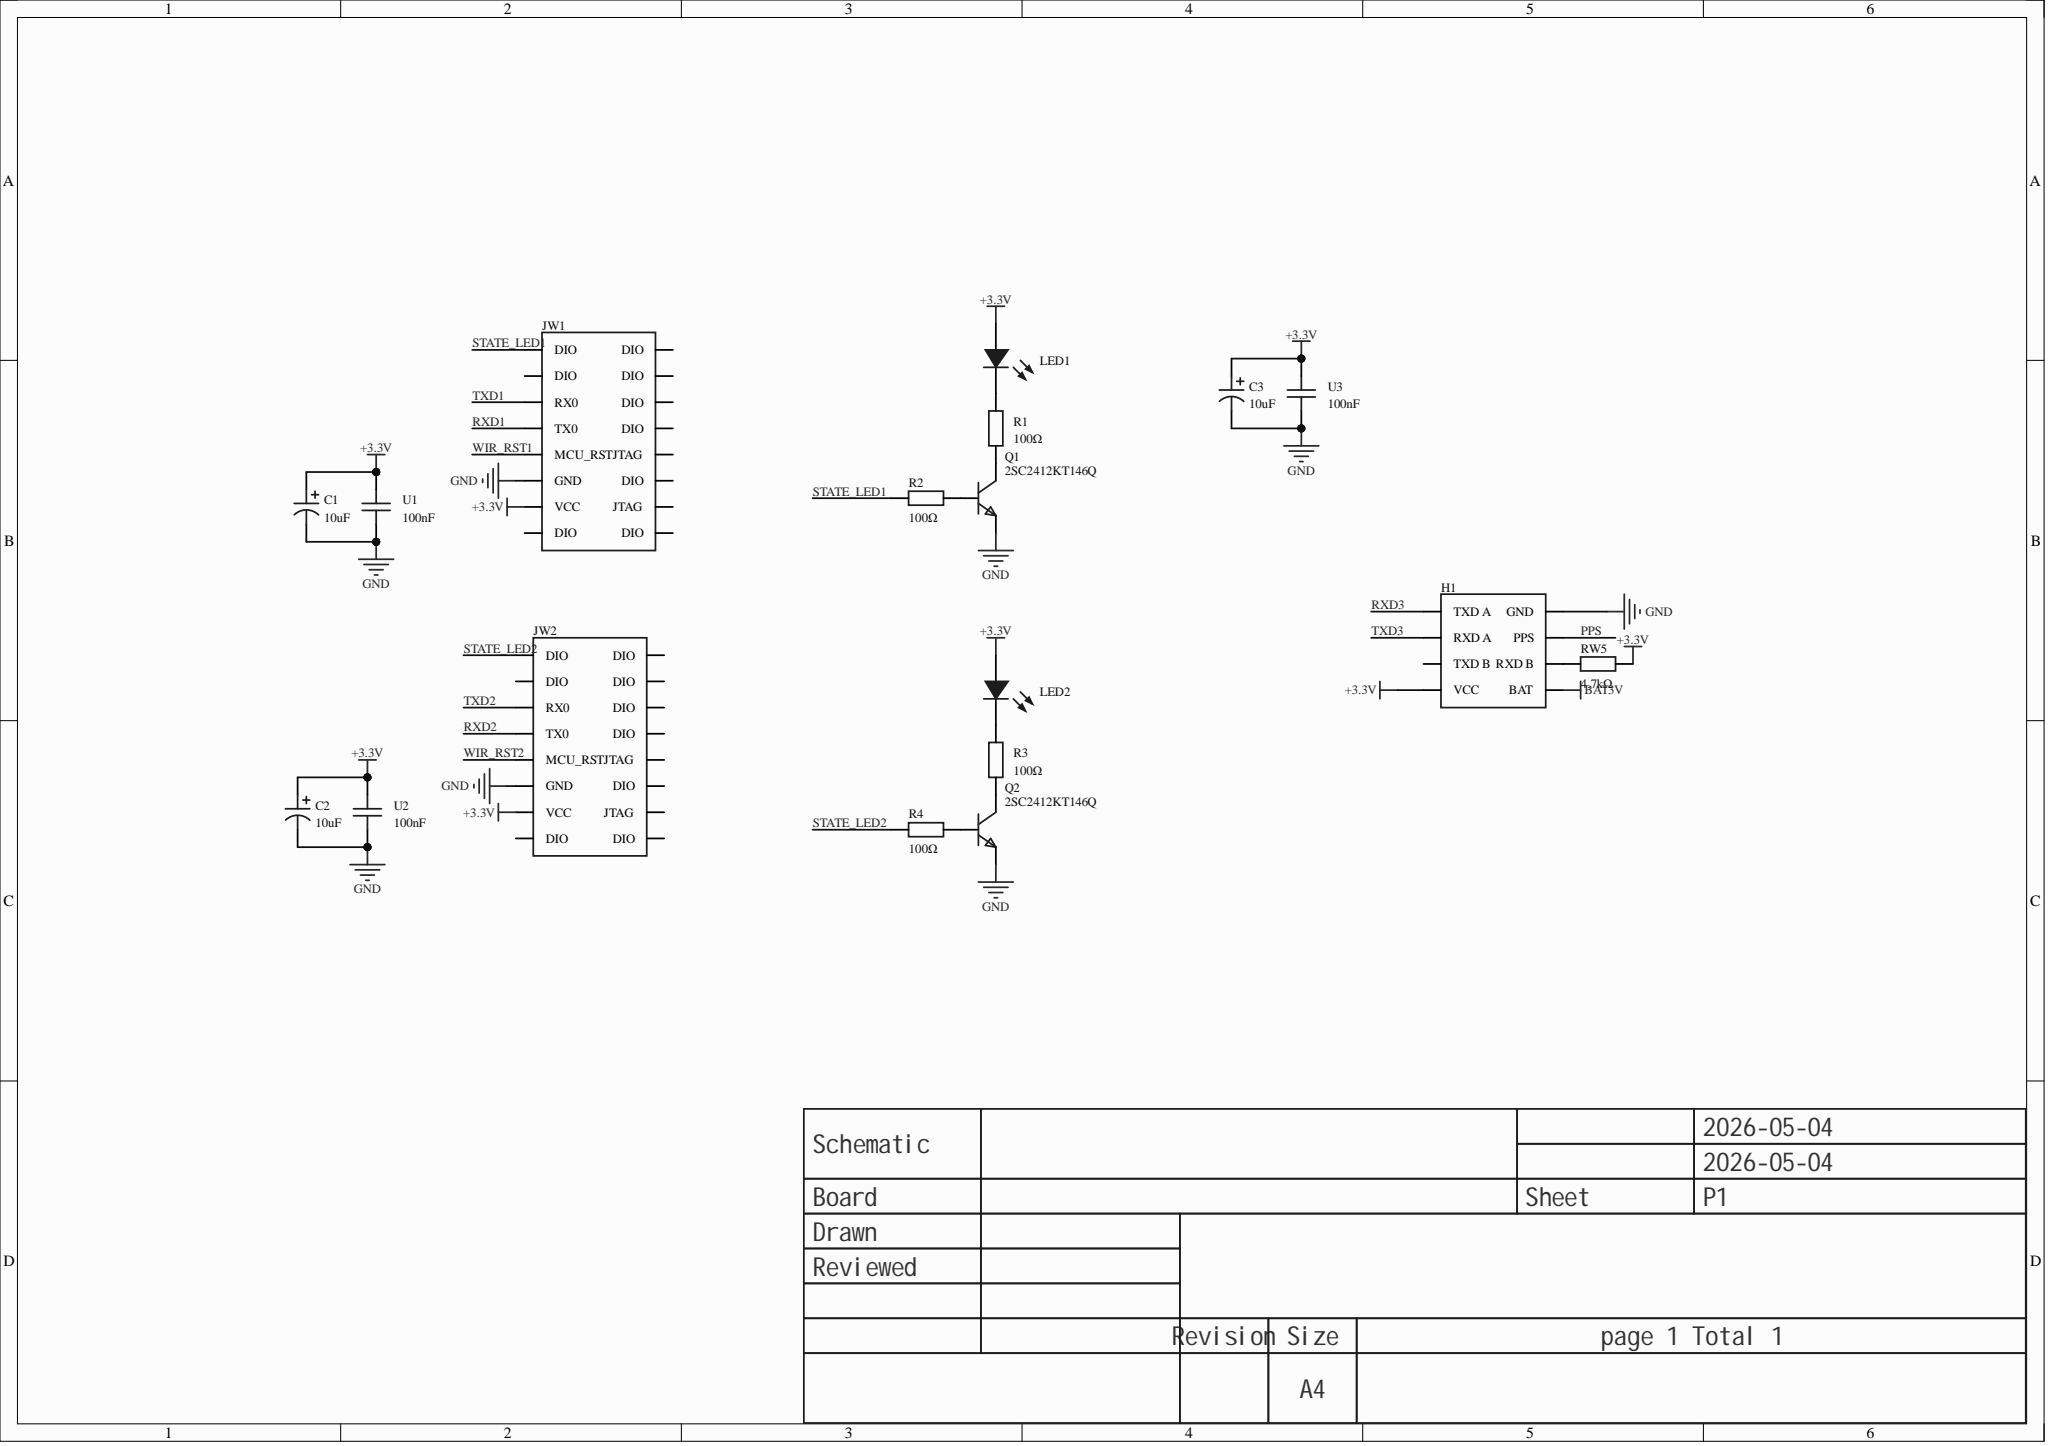Circuit board | Altium Designer | 18 parts | 11 nets
Bill of materials:
Comment,Description,Designator,Footprint,LibRef,Quantity
"10uF","","C1, C2, C3","CAP-TH_BD5.0-P2.00-D0.8-FD-10UF50VC110GL","10UF50VC110GL","3"
"","","H1","HDR-TH_8P-P2.54-V-F-R2-C4-S2.54-1","HDR-F_2.54_2x4","1"
"","","JW1, JW2","HDR-TH_16P-P2.54-V-F-R2-C8-S2.54-1","HDR-F_2.54_2x8","2"
"","","LED1, LED2","LED_TH-3mm","LED_TH-B_3mm","2"
"2SC2412KT146Q","晶体管类型:NPN;集电极电流(Ic):150mA;集射极击穿电压(Vceo):50V;耗散功率(Pd):200mW;直流电流增益(hFE):120@1mA,6V;","Q1, Q2","SOT-346_L2.9-W1.6-P1.90-LS2.8-TR-CW-1","2SC2412KT146Q","2"
"100Ω","","R1, R2, R3, R4","Res_1/8W","Res_AXIAL-1/8W","4"
"4.7kΩ","","RW5","Res_1/8W","Res_AXIAL-1/8W","1"
"100nF","","U1, U2, U3","CAP-TH_L5.0-W2.5-P5.00-D1.0","100nF","3"
Netlist (Protel format):
[
C1
CAP-TH_BD5.0-P2.00-D0.8-FD-10UF50VC110GL
10uF



]
[
C2
CAP-TH_BD5.0-P2.00-D0.8-FD-10UF50VC110GL
10uF



]
[
C3
CAP-TH_BD5.0-P2.00-D0.8-FD-10UF50VC110GL
10uF



]
[
H1
HDR-TH_8P-P2.54-V-F-R2-C4-S2.54-1




]
[
JW1
HDR-TH_16P-P2.54-V-F-R2-C8-S2.54-1




]
[
JW2
HDR-TH_16P-P2.54-V-F-R2-C8-S2.54-1




]
[
LED1
LED_TH-3mm




]
[
LED2
LED_TH-3mm




]
[
Q1
SOT-346_L2.9-W1.6-P1.90-LS2.8-TR-CW-1
2SC2412KT146Q



]
[
Q2
SOT-346_L2.9-W1.6-P1.90-LS2.8-TR-CW-1
2SC2412KT146Q



]
[
R1
Res_1/8W
100Ω



]
[
R2
Res_1/8W
100Ω



]
[
R3
Res_1/8W
100Ω



]
[
R4
Res_1/8W
100Ω



]
[
RW5
Res_1/8W
4.7kΩ



]
[
U1
CAP-TH_L5.0-W2.5-P5.00-D1.0
100nF



]
[
U2
CAP-TH_L5.0-W2.5-P5.00-D1.0
100nF



]
[
U3
CAP-TH_L5.0-W2.5-P5.00-D1.0
100nF



]
(
STATE_LED2
JW2-1
R4-2
)
(
STATE_LED1
JW1-1
R2-2
)
(
NetQ2_3
Q2-3
R3-1
)
(
NetQ2_2
Q2-2
R4-1
)
(
NetQ1_3
Q1-3
R1-1
)
(
NetQ1_2
Q1-2
R2-1
)
(
NetLED2_2
LED2-2
R3-2
)
(
NetLED1_2
LED1-2
R1-2
)
(
NetH1_6
H1-6
RW5-1
)
(
GND
C1-2
C2-2
C3-2
H1-2
JW1-11
JW2-11
Q1-1
Q2-1
U1-2
U2-2
U3-2
)
(
+3.3V
C1-1
C2-1
C3-1
H1-7
JW1-13
JW2-13
LED1-1
LED2-1
RW5-2
U1-1
U2-1
U3-1
)